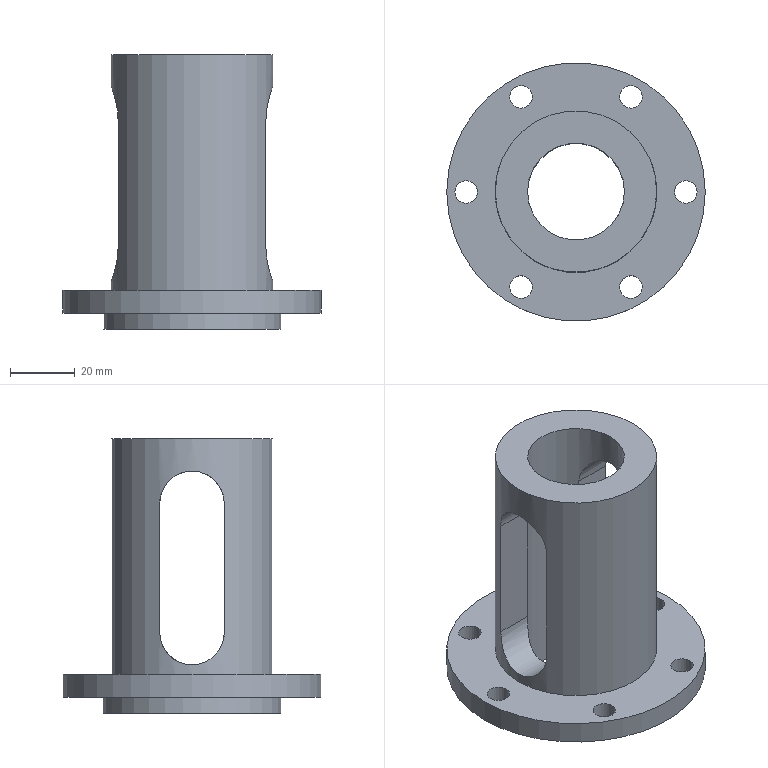NC program | NX | posted with a generic post | part box 80 x 80 x 85 mm
Whole program:
N10 G17 G21 G94 G90
(DRILLING , TOOL : ZXZ)
N12 T01 M6
N14 G54
N16 G17 G0 G90 X-34. Y0. B0. C0. S3000 M3
N18 G43 Z30. H1
N20 G94 G81 G98 Z-6. F200. R-2.
N22 X-17. Y29.445
N24 X17.
N26 X34. Y0.
N28 X17. Y-29.445
N30 X-17.
N32 G80
N34 G0 X-17. Y-29.445 Z30.
N36 M5
(DRILLING_COPY , TOOL : 7.0ZT)
N38 T02 M6
N40 G54
N42 G17 G0 G90 X-34. Y0. B0. C0. S2000 M3
N44 G43 Z30. H2
N46 G94 G83 G98 Z-15.603 F200. Q2. R-2.
N48 X-17. Y29.445
N50 X17.
N52 X34. Y0.
N54 X17. Y-29.445
N56 X-17.
N58 G80
N60 G0 X-17. Y-29.445 Z30.
N62 M5
N64 M2